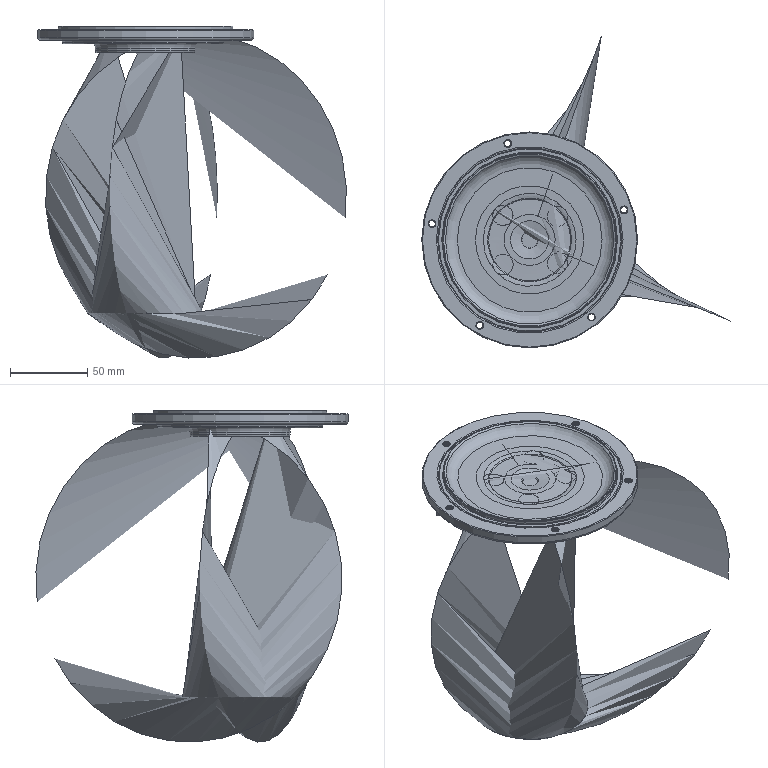NC program | NX | posted with a generic post
Lines 1 to 1953 of 2005, first 1677 of 1941 lines:
N10 G17 G21 G94 G90
(FLOOR_WALL_COPY , TOOL : D63)
N12 T01 M6
N14 G54
N16 G17 G0 G90 X-107.375 Y69.872 S6500 M3
N18 G43 Z30. H1
N20 Z5.
N22 G94 G1 Z2. F1250.
N24 X-101.375
N26 X101.375
N28 Y31.69
N30 X-101.375
N32 Y-6.493
N34 X101.375
N36 Y-44.675
N38 X-101.375
N40 X-107.375
N42 Z5.
N44 G0 Z30.
N46 Y69.872
N48 Z4.
N50 G1 Z1.
N52 X-101.375
N54 X101.375
N56 Y31.69
N58 X-101.375
N60 Y-6.493
N62 X101.375
N64 Y-44.675
N66 X-101.375
N68 X-107.375
N70 Z4.
N72 G0 Z30.
N74 Y69.872
N76 Z3.
N78 G1 Z0.
N80 X-101.375
N82 X101.375
N84 Y31.69
N86 X-101.375
N88 Y-6.493
N90 X101.375
N92 Y-44.675
N94 X-101.375
N96 X-107.375
N98 Z3.
N100 G0 Z30.
N102 M5
(CAVITY_MILL_COPY , TOOL : D10)
N104 T10 M6
N106 G54
N108 G17 G0 G90 X-76.871 Y-18.279 S9500 M3
N110 G43 Z30. H10
N112 Z0.1
N114 G94 G1 Z-0.9 F750.
N116 X-70.871 Y-14.815
N118 G3 X-70.371 Y-13.949 R1.
N120 G1 Y25.577 F3000.
N122 G2 X-25.577 Y70.371 R74.875
N124 G1 X25.577
N126 G2 X70.371 Y25.577 R74.875
N128 G1 Y-25.577
N130 G2 X25.577 Y-70.371 R74.875
N132 G1 X-25.577
N134 G2 X-70.371 Y-25.577 R74.875
N136 G1 Y-13.949
N138 X-63.871
N140 Y24.405
N142 G2 X-24.405 Y63.871 R68.375
N144 G1 X24.405
N146 G2 X63.871 Y24.405 R68.375
N148 G1 Y-24.405
N150 G2 X24.405 Y-63.871 R68.375
N152 G1 X-24.405
N154 G2 X-63.871 Y-24.405 R68.375
N156 G1 Y-13.949
N158 X-57.371
N160 Y23.175
N162 G2 X-23.175 Y57.371 R61.875
N164 G1 X23.175
N166 G2 X57.371 Y23.175 R61.875
N168 G1 Y-23.175
N170 G2 X23.175 Y-57.371 R61.875
N172 G1 X-23.175
N174 G2 X-57.371 Y-23.175 R61.875
N176 G1 Y-13.949
N178 X-50.871
N180 Y21.875
N182 G2 X-21.875 Y50.871 R55.375
N184 G1 X21.875
N186 G2 X50.871 Y21.875 R55.375
N188 G1 Y-21.875
N190 G2 X21.875 Y-50.871 R55.375
N192 G1 X-21.875
N194 G2 X-50.871 Y-21.875 R55.375
N196 G1 Y-13.949
N198 X-44.371
N200 Y20.493
N202 G2 X-20.493 Y44.371 R48.875
N204 G1 X-8.886
N206 Y37.871
N208 G3 X-37.871 Y8.886 R38.9
N210 G1 Y19.011
N212 G2 X-19.011 Y37.871 R42.375
N214 G1 X-8.886
N216 X0. Y39.1
N218 X-8.886 Y37.871
N220 Y44.371
N222 X20.493
N224 G2 X44.371 Y20.493 R48.875
N226 G1 Y8.886
N228 X37.871
N230 G3 X8.886 Y37.871 R38.9
N232 G1 X19.011
N234 G2 X37.871 Y19.011 R42.375
N236 G1 Y8.886
N238 X39.1 Y0.
N240 X37.871 Y8.886
N242 X44.371
N244 Y-20.493
N246 G2 X20.493 Y-44.371 R48.875
N248 G1 X8.886
N250 Y-37.871
N252 G3 X37.871 Y-8.886 R38.9
N254 G1 Y-19.011
N256 G2 X19.011 Y-37.871 R42.375
N258 G1 X8.886
N260 Y-44.371
N262 X-20.493
N264 G2 X-44.371 Y-20.493 R48.875
N266 G1 Y-13.949
N268 X-37.871
N270 Y-8.886
N272 X-39.1 Y0.
N274 X-37.871 Y-8.886
N276 G3 X-8.886 Y-37.871 R38.9
N278 G1 X0. Y-39.1
N280 X-8.886 Y-37.871
N282 X-8.589 Y-36.605
N284 G2 X-36.605 Y8.589 R37.6
N286 X-8.589 Y-36.605 R-37.6
N288 G1 X-8.886 Y-37.871
N290 X-19.011
N292 G2 X-37.871 Y-19.011 R42.375
N294 G1 Y-13.949
N296 G3 X-38.371 Y-13.082 R1.
N298 G1 Z0.1
N300 G0 X-76.871 Y-18.387 Z-0.8
N302 G1 Z-1.8 F750.
N304 X-70.871 Y-14.922
N306 G3 X-70.371 Y-14.056 R1.
N308 G1 Y25.576 F3000.
N310 G2 X-25.576 Y70.371 R74.875
N312 G1 X25.576
N314 G2 X70.371 Y25.576 R74.875
N316 G1 Y-25.576
N318 G2 X25.576 Y-70.371 R74.875
N320 G1 X-25.576
N322 G2 X-70.371 Y-25.576 R74.875
N324 G1 Y-14.056
N326 X-63.871
N328 Y24.405
N330 G2 X-24.405 Y63.871 R68.375
N332 G1 X24.405
N334 G2 X63.871 Y24.405 R68.375
N336 G1 Y-24.405
N338 G2 X24.405 Y-63.871 R68.375
N340 G1 X-24.405
N342 G2 X-63.871 Y-24.405 R68.375
N344 G1 Y-14.056
N346 X-57.371
N348 Y23.174
N350 G2 X-23.174 Y57.371 R61.875
N352 G1 X23.174
N354 G2 X57.371 Y23.174 R61.875
N356 G1 Y-23.174
N358 G2 X23.174 Y-57.371 R61.875
N360 G1 X-23.174
N362 G2 X-57.371 Y-23.174 R61.875
N364 G1 Y-14.056
N366 X-50.871
N368 Y21.875
N370 G2 X-21.875 Y50.871 R55.375
N372 G1 X21.875
N374 G2 X50.871 Y21.875 R55.375
N376 G1 Y-21.875
N378 G2 X21.875 Y-50.871 R55.375
N380 G1 X-21.875
N382 G2 X-50.871 Y-21.875 R55.375
N384 G1 Y-14.056
N386 X-44.371
N388 Y20.493
N390 G2 X-20.493 Y44.371 R48.875
N392 G1 X-9.102
N394 Y37.871
N396 G3 X-37.871 Y9.102 R38.95
N398 G1 Y19.011
N400 G2 X-19.011 Y37.871 R42.375
N402 G1 X-9.102
N404 X0. Y39.12
N406 X-9.102 Y37.871
N408 Y44.371
N410 X20.493
N412 G2 X44.371 Y20.493 R48.875
N414 G1 Y9.102
N416 X37.871
N418 G3 X9.102 Y37.871 R38.95
N420 G1 X19.011
N422 G2 X37.871 Y19.011 R42.375
N424 G1 Y9.102
N426 X39.12 Y0.
N428 X37.871 Y9.102
N430 X44.371
N432 Y-20.493
N434 G2 X20.493 Y-44.371 R48.875
N436 G1 X9.102
N438 Y-37.871
N440 G3 X37.871 Y-9.102 R38.95
N442 G1 Y-19.011
N444 G2 X19.011 Y-37.871 R42.375
N446 G1 X9.102
N448 Y-44.371
N450 X-20.493
N452 G2 X-44.371 Y-20.493 R48.875
N454 G1 Y-14.056
N456 X-37.871
N458 Y-9.102
N460 X-39.12 Y0.
N462 X-37.871 Y-9.102
N464 G3 X-9.102 Y-37.871 R38.95
N466 G1 X0. Y-39.12
N468 X-9.102 Y-37.871
N470 X-8.798 Y-36.607
N472 G2 X-36.607 Y8.798 R37.65
N474 X-8.798 Y-36.607 R-37.65
N476 G1 X-9.102 Y-37.871
N478 X-19.011
N480 G2 X-37.871 Y-19.011 R42.375
N482 G1 Y-14.056
N484 G3 X-38.371 Y-13.19 R1.
N486 G1 Z-0.8
N488 G0 X-76.871 Y-18.388 Z-1.7
N490 G1 Z-2.7 F750.
N492 X-70.871 Y-14.924
N494 G3 X-70.371 Y-14.057 R1.
N496 G1 Y25.576 F3000.
N498 G2 X-25.576 Y70.371 R74.875
N500 G1 X25.576
N502 G2 X70.371 Y25.576 R74.875
N504 G1 Y-25.576
N506 G2 X25.576 Y-70.371 R74.875
N508 G1 X-25.576
N510 G2 X-70.371 Y-25.576 R74.875
N512 G1 Y-14.057
N514 X-63.871
N516 Y24.404
N518 G2 X-24.404 Y63.871 R68.375
N520 G1 X24.404
N522 G2 X63.871 Y24.404 R68.375
N524 G1 Y-24.404
N526 G2 X24.404 Y-63.871 R68.375
N528 G1 X-24.404
N530 G2 X-63.871 Y-24.404 R68.375
N532 G1 Y-14.057
N534 X-57.371
N536 Y23.174
N538 G2 X-23.174 Y57.371 R61.875
N540 G1 X23.174
N542 G2 X57.371 Y23.174 R61.875
N544 G1 Y-23.174
N546 G2 X23.174 Y-57.371 R61.875
N548 G1 X-23.174
N550 G2 X-57.371 Y-23.174 R61.875
N552 G1 Y-14.057
N554 X-50.871
N556 Y21.874
N558 G2 X-21.874 Y50.871 R55.375
N560 G1 X21.874
N562 G2 X50.871 Y21.874 R55.375
N564 G1 Y-21.874
N566 G2 X21.874 Y-50.871 R55.375
N568 G1 X-21.874
N570 G2 X-50.871 Y-21.874 R55.375
N572 G1 Y-14.057
N574 X-44.371
N576 Y20.492
N578 G2 X-20.492 Y44.371 R48.875
N580 G1 X-9.105
N582 Y37.871
N584 G3 X-17.369 Y34.864 R38.951
N586 X-19.724 Y33.588 R38.951
N588 X-21.468 Y32.5 R38.951
N590 X-22.403 Y31.863 R38.951
N592 X-24.645 Y30.163 R38.951
N594 X-30.163 Y24.645 R38.951
N596 X-33.556 Y19.777 R38.951
N598 X-35.962 Y14.962 R38.951
N600 X-36.787 Y12.802 R38.951
N602 X-37.585 Y10.222 R38.951
N604 X-37.871 Y9.105 R38.951
N606 G1 Y19.01
N608 G2 X-19.01 Y37.871 R42.375
N610 G1 X-9.105
N612 X0. Y39.12
N614 X-9.105 Y37.871
N616 Y44.371
N618 X20.492
N620 G2 X44.371 Y20.492 R48.875
N622 G1 Y9.105
N624 X37.871
N626 G3 X13.605 Y36.497 R38.951
N628 X9.105 Y37.871 R38.951
N630 G1 X19.01
N632 G2 X37.871 Y19.01 R42.375
N634 G1 Y9.105
N636 X39.12 Y0.
N638 X37.871 Y9.105
N640 X44.371
N642 Y-20.492
N644 G2 X20.492 Y-44.371 R48.875
N646 G1 X9.105
N648 Y-37.871
N650 G3 X37.871 Y-9.105 R38.951
N652 G1 Y-19.01
N654 G2 X19.01 Y-37.871 R42.375
N656 G1 X9.105
N658 Y-44.371
N660 X-20.492
N662 G2 X-44.371 Y-20.492 R48.875
N664 G1 Y-14.057
N666 X-37.871
N668 Y-9.105
N670 X-39.12 Y0.
N672 X-37.871 Y-9.105
N674 G3 X-9.105 Y-37.871 R38.951
N676 G1 X0. Y-39.12
N678 X-9.105 Y-37.871
N680 X-8.801 Y-36.607
N682 G2 X-29.083 Y-23.911 R37.651
N684 G1 X-29.156 Y-23.822
N686 G2 X-30.8 Y-21.655 R37.651
N688 G1 X-30.9 Y-21.511
N690 G2 X-37.65 Y-0.121 R37.651
N692 X-37.65 Y0.121 R37.651
N694 X16.143 Y34.014 R37.651
N696 G1 X16.243 Y33.967
N698 G2 X-8.801 Y-36.607 R37.651
N700 G1 X-9.105 Y-37.871
N702 X-19.01
N704 G2 X-37.871 Y-19.01 R42.375
N706 G1 Y-14.057
N708 G3 X-38.371 Y-13.191 R1.
N710 G1 Z-1.7
N712 G0 X-76.872 Y-18.597 Z-2.6
N714 G1 Z-3.6 F750.
N716 X-70.872 Y-15.132
N718 G3 X-70.372 Y-14.266 R1.
N720 G1 Y25.575 F3000.
N722 G2 X-25.575 Y70.372 R74.875
N724 G1 X25.575
N726 G2 X70.372 Y25.575 R74.875
N728 G1 Y-25.575
N730 G2 X25.575 Y-70.372 R74.875
N732 G1 X-25.575
N734 G2 X-70.372 Y-25.575 R74.875
N736 G1 Y-14.266
N738 X-63.872
N740 Y24.404
N742 G2 X-24.404 Y63.872 R68.375
N744 G1 X24.404
N746 G2 X63.872 Y24.404 R68.375
N748 G1 Y-24.404
N750 G2 X24.404 Y-63.872 R68.375
N752 G1 X-24.404
N754 G2 X-63.872 Y-24.404 R68.375
N756 G1 Y-14.266
N758 X-57.372
N760 Y23.173
N762 G2 X-23.173 Y57.372 R61.875
N764 G1 X23.173
N766 G2 X57.372 Y23.173 R61.875
N768 G1 Y-23.173
N770 G2 X23.173 Y-57.372 R61.875
N772 G1 X-23.173
N774 G2 X-57.372 Y-23.173 R61.875
N776 G1 Y-14.266
N778 X-50.872
N780 Y21.874
N782 G2 X-21.874 Y50.872 R55.375
N784 G1 X21.874
N786 G2 X50.872 Y21.874 R55.375
N788 G1 Y-21.874
N790 G2 X21.874 Y-50.872 R55.375
N792 G1 X-21.874
N794 G2 X-50.872 Y-21.874 R55.375
N796 G1 Y-14.266
N798 X-44.372
N800 Y20.492
N802 G2 X-20.492 Y44.372 R48.875
N804 G1 X-9.523
N806 Y37.872
N808 G3 X-37.872 Y9.523 R39.051
N810 G1 Y19.01
N812 G2 X-19.01 Y37.872 R42.375
N814 G1 X-9.523
N816 X-4.606 Y38.778
N818 G2 X4.606 Y38.778 R39.051
N820 X4.753 Y39.372 R5.
N822 G1 X-4.753
N824 G2 X-4.606 Y38.778 R5.
N826 G1 X-9.523 Y37.872
N828 Y44.372
N830 X20.492
N832 G2 X44.372 Y20.492 R48.875
N834 G1 Y9.523
N836 X37.872
N838 G3 X9.523 Y37.872 R39.051
N840 G1 X19.01
N842 G2 X37.872 Y19.01 R42.375
N844 G1 Y9.523
N846 X38.778 Y4.606
N848 G2 X38.778 Y-4.606 R39.051
N850 X39.372 Y-4.753 R5.
N852 G1 Y4.753
N854 G2 X38.778 Y4.606 R5.
N856 G1 X37.872 Y9.523
N858 X44.372
N860 Y-20.492
N862 G2 X20.492 Y-44.372 R48.875
N864 G1 X9.523
N866 Y-37.872
N868 G3 X37.872 Y-9.523 R39.051
N870 G1 Y-19.01
N872 G2 X19.01 Y-37.872 R42.375
N874 G1 X9.523
N876 Y-44.372
N878 X-20.492
N880 G2 X-44.372 Y-20.492 R48.875
N882 G1 Y-14.266
N884 X-37.872
N886 Y-9.523
N888 X-38.778 Y-4.606
N890 G2 X-38.778 Y4.606 R39.051
N892 X-39.372 Y4.753 R5.
N894 G1 Y-4.753
N896 G2 X-38.778 Y-4.606 R5.
N898 G1 X-37.872 Y-9.523
N900 G3 X-9.523 Y-37.872 R39.051
N902 G1 X-4.753 Y-39.372
N904 X4.753
N906 G2 X4.606 Y-38.778 R5.
N908 X-4.606 Y-38.778 R39.051
N910 X-4.753 Y-39.372 R5.
N912 G1 X-9.523 Y-37.872
N914 X-9.206 Y-36.611
N916 G2 X-36.611 Y9.206 R37.751
N918 X-9.206 Y-36.611 R-37.751
N920 G1 X-9.523 Y-37.872
N922 X-19.01
N924 G2 X-37.872 Y-19.01 R42.375
N926 G1 Y-14.266
N928 G3 X-38.372 Y-13.4 R1.
N930 G1 Z-2.6
N932 G0 X-76.872 Y-19.041 Z-3.355
N934 G1 Z-4.355 F750.
N936 X-70.872 Y-15.576
N938 G3 X-70.372 Y-14.71 R1.
N940 G1 Y25.575 F3000.
N942 G2 X-25.575 Y70.372 R74.875
N944 G1 X25.575
N946 G2 X70.372 Y25.575 R74.875
N948 G1 Y-25.575
N950 G2 X25.575 Y-70.372 R74.875
N952 G1 X-25.575
N954 G2 X-70.372 Y-25.575 R74.875
N956 G1 Y-14.71
N958 X-63.872
N960 Y24.403
N962 G2 X-24.403 Y63.872 R68.375
N964 G1 X24.403
N966 G2 X63.872 Y24.403 R68.375
N968 G1 Y-24.403
N970 G2 X24.403 Y-63.872 R68.375
N972 G1 X-24.403
N974 G2 X-63.872 Y-24.403 R68.375
N976 G1 Y-14.71
N978 X-57.372
N980 Y23.173
N982 G2 X-23.173 Y57.372 R61.875
N984 G1 X23.173
N986 G2 X57.372 Y23.173 R61.875
N988 G1 Y-23.173
N990 G2 X23.173 Y-57.372 R61.875
N992 G1 X-23.173
N994 G2 X-57.372 Y-23.173 R61.875
N996 G1 Y-14.71
N998 X-50.872
N1000 Y21.873
N1002 G2 X-21.873 Y50.872 R55.375
N1004 G1 X21.873
N1006 G2 X50.872 Y21.873 R55.375
N1008 G1 Y-21.873
N1010 G2 X21.873 Y-50.872 R55.375
N1012 G1 X-21.873
N1014 G2 X-50.872 Y-21.873 R55.375
N1016 G1 Y-14.71
N1018 X-44.372
N1020 Y20.492
N1022 G2 X-20.492 Y44.372 R48.875
N1024 G1 X-10.411
N1026 Y37.872
N1028 G3 X-37.872 Y10.411 R39.277
N1030 G1 Y19.01
N1032 G2 X-19.01 Y37.872 R42.375
N1034 G1 X-10.411
N1036 X-5.516 Y38.888
N1038 G2 X5.516 Y38.888 R39.277
N1040 X5.642 Y39.372 R5.
N1042 G1 X-5.642
N1044 G2 X-5.516 Y38.888 R5.
N1046 G1 X-10.411 Y37.872
N1048 Y44.372
N1050 X20.492
N1052 G2 X44.372 Y20.492 R48.875
N1054 G1 Y10.411
N1056 X37.872
N1058 G3 X10.411 Y37.872 R39.277
N1060 G1 X19.01
N1062 G2 X37.872 Y19.01 R42.375
N1064 G1 Y10.411
N1066 X38.888 Y5.516
N1068 G2 X38.888 Y-5.516 R39.277
N1070 X39.372 Y-5.642 R5.
N1072 G1 Y5.642
N1074 G2 X38.888 Y5.516 R5.
N1076 G1 X37.872 Y10.411
N1078 X44.372
N1080 Y-20.492
N1082 G2 X20.492 Y-44.372 R48.875
N1084 G1 X10.411
N1086 Y-37.872
N1088 G3 X37.872 Y-10.411 R39.277
N1090 G1 Y-19.01
N1092 G2 X19.01 Y-37.872 R42.375
N1094 G1 X10.411
N1096 Y-44.372
N1098 X-20.492
N1100 G2 X-44.372 Y-20.492 R48.875
N1102 G1 Y-14.71
N1104 X-37.872
N1106 Y-10.411
N1108 X-38.888 Y-5.516
N1110 G2 X-38.888 Y5.516 R39.277
N1112 X-39.372 Y5.642 R5.
N1114 G1 Y-5.642
N1116 G2 X-38.888 Y-5.516 R5.
N1118 G1 X-37.872 Y-10.411
N1120 G3 X-10.411 Y-37.872 R39.277
N1122 G1 X-5.642 Y-39.372
N1124 X5.642
N1126 G2 X5.516 Y-38.888 R5.
N1128 X-5.516 Y-38.888 R39.277
N1130 X-5.642 Y-39.372 R5.
N1132 G1 X-10.411 Y-37.872
N1134 X-10.067 Y-36.618
N1136 G2 X-36.618 Y10.067 R37.977
N1138 X-10.067 Y-36.618 R-37.977
N1140 G1 X-10.411 Y-37.872
N1142 X-19.01
N1144 G2 X-37.872 Y-19.01 R42.375
N1146 G1 Y-14.71
N1148 G3 X-38.372 Y-13.844 R1.
N1150 G1 Z-3.355
N1152 G0 X-76.872 Y-19.706 Z-4.111
N1154 G1 Z-5.111 F750.
N1156 X-70.872 Y-16.241
N1158 G3 X-70.372 Y-15.375 R1.
N1160 G1 Y25.574 F3000.
N1162 G2 X-25.574 Y70.372 R74.875
N1164 G1 X25.574
N1166 G2 X70.372 Y25.574 R74.875
N1168 G1 Y-25.574
N1170 G2 X25.574 Y-70.372 R74.875
N1172 G1 X-25.574
N1174 G2 X-70.372 Y-25.574 R74.875
N1176 G1 Y-15.375
N1178 X-63.872
N1180 Y24.403
N1182 G2 X-24.403 Y63.872 R68.375
N1184 G1 X24.403
N1186 G2 X63.872 Y24.403 R68.375
N1188 G1 Y-24.403
N1190 G2 X24.403 Y-63.872 R68.375
N1192 G1 X-24.403
N1194 G2 X-63.872 Y-24.403 R68.375
N1196 G1 Y-15.375
N1198 X-57.372
N1200 Y23.173
N1202 G2 X-23.173 Y57.372 R61.875
N1204 G1 X23.173
N1206 G2 X57.372 Y23.173 R61.875
N1208 G1 Y-23.173
N1210 G2 X23.173 Y-57.372 R61.875
N1212 G1 X-23.173
N1214 G2 X-57.372 Y-23.173 R61.875
N1216 G1 Y-15.375
N1218 X-50.872
N1220 Y21.873
N1222 G2 X-21.873 Y50.872 R55.375
N1224 G1 X21.873
N1226 G2 X50.872 Y21.873 R55.375
N1228 G1 Y-21.873
N1230 G2 X21.873 Y-50.872 R55.375
N1232 G1 X-21.873
N1234 G2 X-50.872 Y-21.873 R55.375
N1236 G1 Y-15.375
N1238 X-44.372
N1240 Y20.491
N1242 G2 X-20.491 Y44.372 R48.875
N1244 G1 X-11.742
N1246 Y37.872
N1248 G3 X-37.872 Y11.742 R39.65
N1250 G1 X-39.267 Y6.206
N1252 X-37.872 Y11.742
N1254 Y19.009
N1256 G2 X-19.009 Y37.872 R42.375
N1258 G1 X-11.742
N1260 X-6.206 Y39.267
N1262 X-11.742 Y37.872
N1264 Y44.372
N1266 X20.491
N1268 G2 X44.372 Y20.491 R48.875
N1270 G1 Y11.742
N1272 X37.872
N1274 G3 X11.742 Y37.872 R39.65
N1276 G1 X6.206 Y39.267
N1278 X11.742 Y37.872
N1280 X19.009
N1282 G2 X37.872 Y19.009 R42.375
N1284 G1 Y11.742
N1286 X39.267 Y6.206
N1288 X37.872 Y11.742
N1290 X44.372
N1292 Y-20.491
N1294 G2 X20.491 Y-44.372 R48.875
N1296 G1 X11.742
N1298 Y-37.872
N1300 G3 X37.872 Y-11.742 R39.65
N1302 G1 X39.267 Y-6.206
N1304 X37.872 Y-11.742
N1306 Y-19.009
N1308 G2 X19.009 Y-37.872 R42.375
N1310 G1 X11.742
N1312 X6.206 Y-39.267
N1314 X11.742 Y-37.872
N1316 Y-44.372
N1318 X-20.491
N1320 G2 X-44.372 Y-20.491 R48.875
N1322 G1 Y-15.375
N1324 X-37.872
N1326 Y-11.742
N1328 X-39.267 Y-6.206
N1330 X-37.872 Y-11.742
N1332 G3 X-11.742 Y-37.872 R39.65
N1334 G1 X-6.206 Y-39.267
N1336 X-11.742 Y-37.872
N1338 X-11.357 Y-36.63
N1340 G2 X-36.63 Y11.357 R38.35
N1342 X-11.357 Y-36.63 R-38.35
N1344 G1 X-11.742 Y-37.872
N1346 X-19.009
N1348 G2 X-37.872 Y-19.009 R42.375
N1350 G1 Y-15.375
N1352 G3 X-38.372 Y-14.509 R1.
N1354 G1 Z-4.111
N1356 G0 X-76.198 Y-23.956 Z-4.866
N1358 G1 Z-5.866 F750.
N1360 X-70.872 Y-20.882
N1362 G3 X-70.372 Y-20.016 R1.
N1364 G1 Y25.574 F3000.
N1366 G2 X-25.574 Y70.372 R74.875
N1368 G1 X25.574
N1370 G2 X70.372 Y25.574 R74.875
N1372 G1 Y-25.574
N1374 G2 X25.574 Y-70.372 R74.875
N1376 G1 X-25.574
N1378 G2 X-70.372 Y-25.574 R74.875
N1380 G1 Y-20.016
N1382 X-63.872
N1384 Y24.403
N1386 G2 X-24.403 Y63.872 R68.375
N1388 G1 X-16.859
N1390 Y57.372
N1392 G3 X-57.372 Y16.859 R59.798
N1394 G1 X-58.776 Y11.531
N1396 X-57.372 Y16.859
N1398 Y23.172
N1400 G2 X-23.172 Y57.372 R61.875
N1402 G1 X-16.859
N1404 X-11.531 Y58.776
N1406 X-16.859 Y57.372
N1408 Y63.872
N1410 X24.403
N1412 G2 X63.872 Y24.403 R68.375
N1414 G1 Y16.859
N1416 X57.372
N1418 G3 X16.859 Y57.372 R59.798
N1420 G1 X11.531 Y58.776
N1422 X16.859 Y57.372
N1424 X23.172
N1426 G2 X57.372 Y23.172 R61.875
N1428 G1 Y16.859
N1430 X58.776 Y11.531
N1432 X57.372 Y16.859
N1434 X63.872
N1436 Y-24.403
N1438 G2 X24.403 Y-63.872 R68.375
N1440 G1 X16.859
N1442 Y-57.372
N1444 G3 X57.372 Y-16.859 R59.798
N1446 G1 X58.776 Y-11.531
N1448 X57.372 Y-16.859
N1450 Y-23.172
N1452 G2 X23.172 Y-57.372 R61.875
N1454 G1 X16.859
N1456 X11.531 Y-58.776
N1458 X16.859 Y-57.372
N1460 Y-63.872
N1462 X-24.403
N1464 G2 X-63.872 Y-24.403 R68.375
N1466 G1 Y-20.016
N1468 X-57.372
N1470 Y-16.859
N1472 X-58.776 Y-11.531
N1474 X-57.372 Y-16.859
N1476 G3 X-16.859 Y-57.372 R59.798
N1478 G1 X-11.531 Y-58.776
N1480 X-16.859 Y-57.372
N1482 X-16.492 Y-56.125
N1484 G2 X-56.125 Y16.492 R58.498
N1486 X-16.492 Y-56.125 R-58.498
N1488 G1 X-16.859 Y-57.372
N1490 X-23.172
N1492 G2 X-57.372 Y-23.172 R61.875
N1494 G1 Y-20.016
N1496 G3 X-57.872 Y-19.15 R1.
N1498 G1 Z-4.866
N1500 G0 X-75.981 Y-24.636 Z-5.622
N1502 G1 Z-6.622 F750.
N1504 X-70.872 Y-21.687
N1506 G3 X-70.372 Y-20.821 R1.
N1508 G1 Y25.573 F3000.
N1510 G2 X-25.573 Y70.372 R74.875
N1512 G1 X25.573
N1514 G2 X70.372 Y25.573 R74.875
N1516 G1 Y-25.573
N1518 G2 X25.573 Y-70.372 R74.875
N1520 G1 X-25.573
N1522 G2 X-70.372 Y-25.573 R74.875
N1524 G1 Y-20.821
N1526 X-63.872
N1528 Y24.402
N1530 G2 X-24.402 Y63.872 R68.375
N1532 G1 X-18.47
N1534 Y57.372
N1536 G3 X-57.372 Y18.47 R60.272
N1538 G1 X-58.817 Y13.423
N1540 X-57.372 Y18.47
N1542 Y23.172
N1544 G2 X-23.172 Y57.372 R61.875
N1546 G1 X-18.47
N1548 X-13.423 Y58.817
N1550 X-18.47 Y57.372
N1552 Y63.872
N1554 X24.402
N1556 G2 X63.872 Y24.402 R68.375
N1558 G1 Y18.47
N1560 X57.372
N1562 G3 X18.47 Y57.372 R60.272
N1564 G1 X13.423 Y58.817
N1566 X18.47 Y57.372
N1568 X23.172
N1570 G2 X57.372 Y23.172 R61.875
N1572 G1 Y18.47
N1574 X58.817 Y13.423
N1576 X57.372 Y18.47
N1578 X63.872
N1580 Y-24.402
N1582 G2 X24.402 Y-63.872 R68.375
N1584 G1 X18.47
N1586 Y-57.372
N1588 G3 X57.372 Y-18.47 R60.272
N1590 G1 X58.817 Y-13.423
N1592 X57.372 Y-18.47
N1594 Y-23.172
N1596 G2 X23.172 Y-57.372 R61.875
N1598 G1 X18.47
N1600 X13.423 Y-58.817
N1602 X18.47 Y-57.372
N1604 Y-63.872
N1606 X-24.402
N1608 G2 X-63.872 Y-24.402 R68.375
N1610 G1 Y-20.821
N1612 X-57.372
N1614 Y-18.47
N1616 X-58.817 Y-13.423
N1618 X-57.372 Y-18.47
N1620 G3 X-18.47 Y-57.372 R60.272
N1622 G1 X-13.423 Y-58.817
N1624 X-18.47 Y-57.372
N1626 X-18.071 Y-56.135
N1628 G2 X-56.135 Y18.071 R58.972
N1630 X-18.071 Y-56.135 R-58.972
N1632 G1 X-18.47 Y-57.372
N1634 X-23.172
N1636 G2 X-57.372 Y-23.172 R61.875
N1638 G1 Y-20.821
N1640 G3 X-57.872 Y-19.955 R1.
N1642 G1 Z-5.622
N1644 G0 X-75.943 Y-24.754 Z-6.414
N1646 G1 Z-7.414 F750.
N1648 X-70.872 Y-21.827
N1650 G3 X-70.372 Y-20.96 R1.
N1652 G1 Y25.573 F3000.
N1654 G2 X-25.573 Y70.372 R74.875
N1656 G1 X25.573
N1658 G2 X70.372 Y25.573 R74.875
N1660 G1 Y-25.573
N1662 G2 X25.573 Y-70.372 R74.875
N1664 G1 X-25.573
N1666 G2 X-70.372 Y-25.573 R74.875
N1668 G1 Y-20.96
N1670 X-63.872
N1672 Y24.402
N1674 G2 X-24.402 Y63.872 R68.375
N1676 G1 X-18.75
N1678 Y57.372
N1680 G3 X-57.372 Y18.75 R60.359
N1682 G1 X-58.824 Y13.743
N1684 X-57.372 Y18.75
N1686 Y23.171
N1688 G2 X-23.171 Y57.372 R61.875
N1690 G1 X-18.75
N1692 X-13.743 Y58.824
N1694 X-18.75 Y57.372
N1696 Y63.872
N1698 X24.402
N1700 G2 X63.872 Y24.402 R68.375
N1702 G1 Y18.75
N1704 X57.372
N1706 G3 X18.75 Y57.372 R60.359
N1708 G1 X13.743 Y58.824
N1710 X18.75 Y57.372
N1712 X23.171
N1714 G2 X57.372 Y23.171 R61.875
N1716 G1 Y18.75
N1718 X58.824 Y13.743
N1720 X57.372 Y18.75
N1722 X63.872
N1724 Y-24.402
N1726 G2 X24.402 Y-63.872 R68.375
N1728 G1 X18.75
N1730 Y-57.372
N1732 G3 X57.372 Y-18.75 R60.359
N1734 G1 X58.824 Y-13.743
N1736 X57.372 Y-18.75
N1738 Y-23.171
N1740 G2 X23.171 Y-57.372 R61.875
N1742 G1 X18.75
N1744 X13.743 Y-58.824
N1746 X18.75 Y-57.372
N1748 Y-63.872
N1750 X-24.402
N1752 G2 X-63.872 Y-24.402 R68.375
N1754 G1 Y-20.96
N1756 X-57.372
N1758 Y-18.75
N1760 X-58.824 Y-13.743
N1762 X-57.372 Y-18.75
N1764 G3 X-18.75 Y-57.372 R60.359
N1766 G1 X-13.743 Y-58.824
N1768 X-18.75 Y-57.372
N1770 X-18.346 Y-56.137
N1772 G2 X-56.137 Y18.346 R59.059
N1774 X-18.346 Y-56.137 R-59.059
N1776 G1 X-18.75 Y-57.372
N1778 X-23.171
N1780 G2 X-57.372 Y-23.171 R61.875
N1782 G1 Y-20.96
N1784 G3 X-57.872 Y-20.094 R1.
N1786 G1 Z-6.414
N1788 G0 X-75.626 Y-25.705 Z-6.957
N1790 G1 Z-7.957 F750.
N1792 X-70.873 Y-22.961
N1794 G3 X-70.373 Y-22.095 R1.
N1796 G1 Y25.573 F3000.
N1798 G2 X-25.573 Y70.373 R74.875
N1800 G1 X25.573
N1802 G2 X70.373 Y25.573 R74.875
N1804 G1 Y-25.573
N1806 G2 X25.573 Y-70.373 R74.875
N1808 G1 X-25.573
N1810 G2 X-70.373 Y-25.573 R74.875
N1812 G1 Y-22.095
N1814 X-63.873
N1816 Y24.401
N1818 G2 X-24.401 Y63.873 R68.375
N1820 G1 X-21.018
N1822 Y57.373
N1824 G3 X-57.373 Y21.018 R61.101
N1826 G1 Y23.171
N1828 G2 X-23.171 Y57.373 R61.875
N1830 G1 X-21.018
N1832 Y63.873
N1834 X24.401
N1836 G2 X63.873 Y24.401 R68.375
N1838 G1 Y21.018
N1840 X57.373
N1842 G3 X21.018 Y57.373 R61.101
N1844 G1 X23.171
N1846 G2 X57.373 Y23.171 R61.875
N1848 G1 Y21.018
N1850 X63.873
N1852 Y-24.401
N1854 G2 X24.401 Y-63.873 R68.375
N1856 G1 X21.018
N1858 Y-57.373
N1860 G3 X57.373 Y-21.018 R61.101
N1862 G1 Y-23.171
N1864 G2 X23.171 Y-57.373 R61.875
N1866 G1 X21.018
N1868 Y-63.873
N1870 X-24.401
N1872 G2 X-63.873 Y-24.401 R68.375
N1874 G1 Y-22.095
N1876 X-57.373
N1878 Y-21.018
N1880 G3 X-21.018 Y-57.373 R61.101
N1882 G1 X-20.571 Y-56.152
N1884 G2 X-56.152 Y20.571 R59.801
N1886 X-20.571 Y-56.152 R-59.801
N1888 G1 X-21.018 Y-57.373
N1890 X-23.171
N1892 G2 X-57.373 Y-23.171 R61.875
N1894 G1 Y-22.095
N1896 G3 X-57.873 Y-21.229 R1.
N1898 G1 Z-6.957
N1900 G0 X-75.923 Y-24.812 Z-7.17
N1902 G1 Z-8.17 F750.
N1904 X-70.684 Y-23.1
N1906 G3 X-70.467 Y-22.124 R1.
N1908 G2 X-22.124 Y70.467 R73.858 F3000.
N1910 X-70.467 Y-22.124 R-73.858
N1912 G3 X-71.203 Y-21.448 R1.
N1914 G1 X-76.873 Y-20.183
N1916 Z-7.17
N1918 G0 Y-29.25 Z-7.875
N1920 G1 Z-8.875 F750.
N1922 X-71.442 Y-23.338
N1924 G3 X-71.224 Y-22.362 R1.
N1926 G2 X-22.362 Y71.224 R74.652 F3000.
N1928 X-71.224 Y-22.362 R-74.652
N1930 G3 X-71.961 Y-21.686 R1.
N1932 G1 X-76.873 Y-20.59
N1934 Z-7.875
N1936 G0 Z30.
N1938 X29.473 Y-30.052
N1940 Z-4.111
N1942 G1 X31.613 Y-27.871 Z-4.271 F750.
N1944 X34.39 Y-24.361 Z-4.506
N1946 X36.78 Y-20.576 Z-4.74
N1948 X38.755 Y-16.559 Z-4.975
N1950 X40.293 Y-12.356 Z-5.209
N1952 X41.376 Y-8.013 Z-5.444
N1954 X41.862 Y-4.87 Z-5.61
N1956 X42.114 Y-1.59 Z-5.783
N1958 Y0. Z-5.866
N1960 G3 X0. Y42.114 R42.114 F3000.
N1962 X42.114 Y0. R-42.114
N1964 G1 X46.614
N1966 G3 X-29.207 Y-36.33 R-46.614
N1968 G1 X-24.386 Y-30.333
N1970 G2 X-30.333 Y24.386 R38.92
N1972 X-24.386 Y-30.333 R-38.92
N1974 G1 X-29.207 Y-36.33
N1976 G3 X46.614 Y0. R46.614
N1978 X46.114 Y0.866 R1.
N1980 G1 Z-4.866
N1982 G0 Z30.
N1984 X-29.656 Y26.524
N1986 Z-4.866
N1988 G1 X-28.742 Y27.586 Z-4.94 F750.
N1990 X-25.612 Y30.514 Z-5.164
N1992 X-22.186 Y33.088 Z-5.389
N1994 X-19.554 Y34.709 Z-5.551
N1996 X-16.179 Y36.405 Z-5.749
N1998 X-12.658 Y37.774 Z-5.947
N2000 X-9.024 Y38.803 Z-6.145
N2002 X-5.309 Y39.483 Z-6.343
N2004 X-1.546 Y39.808 Z-6.541
N2006 X0. Z-6.622
N2008 G2 X39.808 Y0. R39.808 F3000.
N2010 X0. Y39.808 R-39.808
N2012 G1 Y43.854
N2014 G3 X-43.854 Y0. R43.854
N2016 X0. Y43.854 R-43.854
N2018 X-0.866 Y43.354 R1.
N2020 G1 Z-5.622
N2022 G0 Z30.
N2024 X4.327 Y2.316
N2026 Z1.
N2028 G1 X4.229 Y2.553 Z0.987 F750.
N2030 X3.264 Y3.708 Z0.908
N2032 X1.997 Y4.519 Z0.829
N2034 X0.544 Y4.91 Z0.75
N2036 X-0.544 Z0.693
N2038 X-1.385 Y4.742 Z0.648
N2040 X-2.185 Y4.43 Z0.603
N2042 X-3.101 Y3.845 Z0.546
N2044 X-4.102 Y2.752 Z0.468
N2046 X-4.734 Y1.411 Z0.391
N2048 X-4.94 Y-0.057 Z0.313
N2050 X-4.7 Y-1.52 Z0.235
N2052 X-4.038 Y-2.846 Z0.158
N2054 X-3.011 Y-3.916 Z0.08
N2056 X-2.082 Y-4.48 Z0.023
N2058 X-0.743 Y-4.884 Z-0.05
N2060 X0.654 Y-4.896 Z-0.124
N2062 X2. Y-4.517 Z-0.197
N2064 X3.185 Y-3.776 Z-0.27
N2066 X4.116 Y-2.732 Z-0.343
N2068 X4.716 Y-1.47 Z-0.417
N2070 X4.924 Y-0.403 Z-0.474
N2072 X4.939 Y0.083 Z-0.499
N2074 X4.802 Y1.161 Z-0.556
N2076 X4.229 Y2.553 Z-0.635
N2078 X3.264 Y3.708 Z-0.714
N2080 X1.997 Y4.519 Z-0.793
N2082 X0.544 Y4.91 Z-0.872
N2084 X0. Z-0.9
N2086 Y0.41
N2088 G3 X-0.41 Y0. R0.41 F3000.
N2090 X0. Y0.41 R-0.41
N2092 G1 Y4.91
N2094 G3 X-4.91 Y0. R4.91
N2096 X0. Y4.91 R-4.91
N2098 G1 Y11.41
N2100 G3 X-11.41 Y0. R11.41
N2102 X0. Y11.41 R-11.41
N2104 G1 Y17.91
N2106 G3 X-17.91 Y0. R17.91
N2108 X0. Y17.91 R-17.91
N2110 G1 Y24.41
N2112 G3 X-24.41 Y0. R24.41
N2114 X0. Y24.41 R-24.41
N2116 X-0.866 Y23.91 R1.
N2118 G1 Z0.1
N2120 G0 Z30.
N2122 X4.327 Y2.316
N2124 Z0.1
N2126 G1 X4.229 Y2.553 Z0.087 F750.
N2128 X3.264 Y3.708 Z0.008
N2130 X1.997 Y4.519 Z-0.071
N2132 X0.544 Y4.91 Z-0.15
N2134 X-0.544 Z-0.207
N2136 X-1.385 Y4.742 Z-0.252
N2138 X-2.185 Y4.43 Z-0.297
N2140 X-3.101 Y3.845 Z-0.354
N2142 X-4.102 Y2.752 Z-0.432
N2144 X-4.734 Y1.411 Z-0.509
N2146 X-4.94 Y-0.057 Z-0.587
N2148 X-4.7 Y-1.52 Z-0.665
N2150 X-4.038 Y-2.846 Z-0.742
N2152 X-3.011 Y-3.916 Z-0.82
N2154 X-2.082 Y-4.48 Z-0.877
N2156 X-0.743 Y-4.884 Z-0.95
N2158 X0.654 Y-4.896 Z-1.024
N2160 X2. Y-4.517 Z-1.097
N2162 X3.185 Y-3.776 Z-1.17
N2164 X4.116 Y-2.732 Z-1.243
N2166 X4.716 Y-1.47 Z-1.317
N2168 X4.924 Y-0.403 Z-1.374
N2170 X4.939 Y0.083 Z-1.399
N2172 X4.802 Y1.161 Z-1.456
N2174 X4.229 Y2.553 Z-1.535
N2176 X3.264 Y3.708 Z-1.614
N2178 X1.997 Y4.519 Z-1.693
N2180 X0.544 Y4.91 Z-1.772
N2182 X0. Z-1.8
N2184 Y0.41
N2186 G3 X-0.41 Y0. R0.41 F3000.
N2188 X0. Y0.41 R-0.41
N2190 G1 Y4.91
N2192 G3 X-4.91 Y0. R4.91
N2194 X0. Y4.91 R-4.91
N2196 G1 Y11.41
N2198 G3 X-11.41 Y0. R11.41
N2200 X0. Y11.41 R-11.41
N2202 G1 Y17.91
N2204 G3 X-17.91 Y0. R17.91
N2206 X0. Y17.91 R-17.91
N2208 G1 Y24.41
N2210 G3 X-24.41 Y0. R24.41
N2212 X0. Y24.41 R-24.41
N2214 X-0.866 Y23.91 R1.
N2216 G1 Z-0.8
N2218 G0 X4.327 Y2.316
N2220 G1 X4.229 Y2.553 Z-0.813 F750.
N2222 X3.264 Y3.708 Z-0.892
N2224 X1.997 Y4.519 Z-0.971
N2226 X0.544 Y4.91 Z-1.05
N2228 X-0.544 Z-1.107
N2230 X-1.385 Y4.742 Z-1.152
N2232 X-2.185 Y4.43 Z-1.197
N2234 X-3.101 Y3.845 Z-1.254
N2236 X-4.102 Y2.752 Z-1.332
N2238 X-4.734 Y1.411 Z-1.409
N2240 X-4.94 Y-0.057 Z-1.487
N2242 X-4.7 Y-1.52 Z-1.565
N2244 X-4.038 Y-2.846 Z-1.642
N2246 X-3.011 Y-3.916 Z-1.72
N2248 X-2.082 Y-4.48 Z-1.777
N2250 X-0.743 Y-4.884 Z-1.85
N2252 X0.654 Y-4.896 Z-1.924
N2254 X2. Y-4.517 Z-1.997
N2256 X3.185 Y-3.776 Z-2.07
N2258 X4.116 Y-2.732 Z-2.143
N2260 X4.716 Y-1.47 Z-2.217
N2262 X4.924 Y-0.403 Z-2.274
N2264 X4.939 Y0.083 Z-2.299
N2266 X4.802 Y1.161 Z-2.356
N2268 X4.229 Y2.553 Z-2.435
N2270 X3.264 Y3.708 Z-2.514
N2272 X1.997 Y4.519 Z-2.593
N2274 X0.544 Y4.91 Z-2.672
N2276 X0. Z-2.7
N2278 Y0.41
N2280 G3 X-0.41 Y0. R0.41 F3000.
N2282 X0. Y0.41 R-0.41
N2284 G1 Y4.91
N2286 G3 X-4.91 Y0. R4.91
N2288 X0. Y4.91 R-4.91
N2290 G1 Y11.41
N2292 G3 X-11.41 Y0. R11.41
N2294 X0. Y11.41 R-11.41
N2296 G1 Y17.91
N2298 G3 X-17.91 Y0. R17.91
N2300 X0. Y17.91 R-17.91
N2302 G1 Y24.41
N2304 G3 X-24.41 Y0. R24.41
N2306 X0. Y24.41 R-24.41
N2308 X-0.866 Y23.91 R1.
N2310 G1 Z-1.7
N2312 G0 X0.808 Y4.446
N2314 G1 X0.76 Y4.462 Z-1.703 F750.
N2316 X-0.581 Y4.489 Z-1.773
N2318 X-1.872 Y4.121 Z-1.843
N2320 X-2.763 Y3.585 Z-1.898
N2322 X-3.609 Y2.731 Z-1.961
N2324 X-4.201 Y1.685 Z-2.024
N2326 X-4.496 Y0.52 Z-2.087
N2328 Y-0.52 Z-2.141
N2330 X-4.221 Y-1.634 Z-2.201
N2332 X-3.675 Y-2.642 Z-2.262
N2334 X-2.893 Y-3.481 Z-2.322
N2336 X-2.021 Y-4.05 Z-2.376
N2338 X-0.839 Y-4.448 Z-2.442
N2340 X0.406 Y-4.508 Z-2.507
N2342 X1.621 Y-4.226 Z-2.572
N2344 X2.713 Y-3.623 Z-2.638
N2346 X3.599 Y-2.745 Z-2.703
N2348 X4.211 Y-1.659 Z-2.768
N2350 X4.479 Y-0.654 Z-2.823
N2352 X4.526 Y-0.083 Z-2.853
N2354 X4.425 Y0.952 Z-2.907
N2356 X3.951 Y2.208 Z-2.978
N2358 X3.131 Y3.269 Z-3.048
N2360 X2.035 Y4.043 Z-3.118
N2362 X0.76 Y4.462 Z-3.189
N2364 X-0.581 Y4.489 Z-3.259
N2366 X-1.872 Y4.121 Z-3.329
N2368 X-2.763 Y3.585 Z-3.384
N2370 X-3.609 Y2.731 Z-3.447
N2372 X-4.201 Y1.685 Z-3.51
N2374 X-4.496 Y0.52 Z-3.573
N2376 Y0. Z-3.6
N2378 G3 X0. Y-4.496 R4.496 F3000.
N2380 X-4.496 Y0. R-4.496
N2382 G1 X-10.996
N2384 G3 X0. Y-10.996 R10.996
N2386 X-10.996 Y0. R-10.996
N2388 G1 X-17.496
N2390 G3 X0. Y-17.496 R17.496
N2392 X-17.496 Y0. R-17.496
N2394 G1 X-23.996
N2396 G3 X0. Y-23.996 R23.996
N2398 X-23.996 Y0. R-23.996
N2400 X-23.496 Y-0.866 R1.
N2402 G1 Z-2.6
N2404 G0 X-0.75 Y-5.464
N2406 G1 X-0.579 Y-5.647 Z-2.613 F750.
N2408 X0. Y-6.449 Z-2.665
N2410 X0.191 Y-6.187 Z-2.682
N2412 X0.845 Y-5.367 Z-2.737
N2414 X1.34 Y-4.839 Z-2.775
N2416 X2.068 Y-4.066 Z-2.831
N2418 X3.257 Y-3.065 Z-2.912
N2420 X4.055 Y-1.886 Z-2.987
N2422 X4.442 Y-0.517 Z-3.061
N2424 Y0.517 Z-3.115
N2426 X4.098 Y1.791 Z-3.185
N2428 X3.397 Y2.909 Z-3.254
N2430 X2.4 Y3.774 Z-3.323
N2432 X1.195 Y4.31 Z-3.392
N2434 X-0.115 Y4.471 Z-3.461
N2436 X-1.414 Y4.243 Z-3.53
N2438 X-2.351 Y3.804 Z-3.584
N2440 X-3.361 Y2.95 Z-3.654
N2442 X-4.077 Y1.838 Z-3.723
N2444 X-4.436 Y0.565 Z-3.792
N2446 X-4.408 Y-0.757 Z-3.862
N2448 X-3.994 Y-2.013 Z-3.931
N2450 X-3.23 Y-3.093 Z-4.
N2452 X-2.069 Y-4.053 Z-4.079
N2454 X-0.579 Y-5.647 Z-4.194
N2456 X0. Y-6.449 Z-4.245
N2458 X0.191 Y-6.187 Z-4.262
N2460 X0.845 Y-5.367 Z-4.317
N2462 X1.34 Y-4.839 Z-4.355
N2464 G2 X2.861 Y-3.398 R17.906 F3000.
N2466 G3 X-2.832 Y-3.423 R-4.442
N2468 G2 X0. Y-6.449 R16.295
N2470 X0.393 Y-5.934 R15.538
N2472 X1.34 Y-4.839 R17.906
N2474 G1 X6.08 Y-9.288
N2476 G2 X7.048 Y-8.37 R11.406
N2478 G3 X-6.975 Y-8.431 R-10.942
N2480 G2 X-4.062 Y-12.501 R9.795
N2482 X-3.506 Y-15.527 R8.53
N2484 G1 Y-19.95
N2486 G3 X3.506 Y-19.95 R20.256
N2488 G1 Y-15.52
N2490 G2 X5.476 Y-9.985 R9.038
N2492 X6.08 Y-9.288 R11.406
N2494 G3 X6.202 Y-9.06 R0.5
N2496 G1 Z-3.355
N2498 G0 X3.531 Y2.625
N2500 G1 X3.504 Y2.671 Z-3.358 F750.
N2502 X2.674 Y3.502 Z-3.42
N2504 X1.654 Y4.084 Z-3.481
N2506 X0.517 Y4.376 Z-3.543
N2508 X-0.51 Y4.377 Z-3.597
N2510 X-1.402 Y4.177 Z-3.645
N2512 X-2.33 Y3.739 Z-3.698
N2514 X-3.331 Y2.884 Z-3.767
N2516 X-4.035 Y1.77 Z-3.836
N2518 X-4.378 Y0.499 Z-3.905
N2520 X-4.33 Y-0.817 Z-3.974
N2522 X-3.895 Y-2.061 Z-4.043
N2524 X-3.112 Y-3.12 Z-4.112
N2526 X-2.709 Y-3.437 Z-4.139
N2528 X-1.916 Y-4.066 Z-4.192
N2530 X-0.634 Y-5.342 Z-4.287
N2532 X-0.002 Y-6.131 Z-4.34
N2534 X0.627 Y-5.346 Z-4.393
N2536 X1.914 Y-4.065 Z-4.488
N2538 X2.703 Y-3.442 Z-4.541
N2540 X3.107 Y-3.125 Z-4.568
N2542 X3.723 Y-2.357 Z-4.619
N2544 X4.153 Y-1.472 Z-4.671
N2546 X4.376 Y-0.513 Z-4.722
N2548 Y0. Z-4.749
N2550 Y0.513 Z-4.776
N2552 X4.085 Y1.651 Z-4.838
N2554 X3.504 Y2.671 Z-4.899
N2556 X2.674 Y3.502 Z-4.961
N2558 X1.654 Y4.084 Z-5.022
N2560 X0.517 Y4.376 Z-5.084
N2562 X0.004 Z-5.111
N2564 G3 X-2.709 Y-3.437 R4.376 F3000.
N2566 G2 X-0.002 Y-6.131 R17.035
N2568 X2.703 Y-3.442 R16.842
N2570 G3 X0.004 Y4.376 R4.376
N2572 G1 X0.009 Y10.876
N2574 G3 X-6.732 Y-8.543 R10.876
N2576 G2 X-4.127 Y-11.595 R10.535
N2578 X-3.07 Y-15.682 R8.675
N2580 G1 Y-19.581
N2582 G3 X3.07 Y-19.581 R19.82
N2584 G1 Y-15.675
N2586 G2 X4.638 Y-10.778 R8.641
N2588 X6.732 Y-8.543 R10.342
N2590 G3 X0.009 Y10.876 R10.876
N2592 X-0.858 Y10.377 R1.
N2594 G1 Z-4.111
N2596 G0 X-2.444 Y-3.542
N2598 G1 X-1.805 Y-3.997 Z-4.152 F750.
N2600 X-0.654 Y-5.024 Z-4.233
N2602 X-0.007 Y-5.746 Z-4.284
N2604 X0.552 Y-5.125 Z-4.327
N2606 X1.178 Y-4.568 Z-4.371
N2608 X1.375 Y-4.393 Z-4.385
N2610 X1.578 Y-4.225 Z-4.399
N2612 X2.48 Y-3.52 Z-4.459
N2614 X2.896 Y-3.227 Z-4.486
N2616 X3.639 Y-2.358 Z-4.545
N2618 X4.128 Y-1.325 Z-4.605
N2620 X4.331 Y-0.2 Z-4.665
N2622 X4.294 Y0.308 Z-4.692
N2624 X4.258 Y0.816 Z-4.719
N2626 X3.83 Y2.03 Z-4.786
N2628 X3.065 Y3.065 Z-4.854
N2630 X2.03 Y3.83 Z-4.921
N2632 X0.816 Y4.258 Z-4.988
N2634 X-0.47 Y4.31 Z-5.056
N2636 X-1.715 Y3.981 Z-5.123
N2638 X-2.597 Y3.472 Z-5.177
N2640 X-3.479 Y2.587 Z-5.242
N2642 X-4.072 Y1.488 Z-5.308
N2644 X-4.327 Y0.265 Z-5.373
N2646 X-4.223 Y-0.98 Z-5.439
N2648 X-3.768 Y-2.144 Z-5.504
N2650 X-3.001 Y-3.129 Z-5.57
N2652 X-2.594 Y-3.436 Z-5.596
N2654 X-1.805 Y-3.997 Z-5.647
N2656 X-0.654 Y-5.024 Z-5.728
N2658 X-0.007 Y-5.746 Z-5.779
N2660 X0.552 Y-5.125 Z-5.822
N2662 X1.176 Y-4.57 Z-5.866
N2664 X1.178 Y-4.568 F3000.
N2666 G2 X1.578 Y-4.225 R15.021
N2668 G1 X2.48 Y-3.52
N2670 G3 X4.294 Y0.308 R4.305
N2672 X-2.594 Y-3.436 R-4.305
N2674 G2 X-0.007 Y-5.746 R15.619
N2676 X1.176 Y-4.57 R15.021
N2678 G1 X5.495 Y-9.428
N2680 G2 X5.671 Y-9.276 R8.521
N2682 G1 X6.408 Y-8.7
N2684 G3 X-6.409 Y-8.7 R-10.805
N2686 G2 X-3.351 Y-12.368 R9.119
N2688 X-2.634 Y-15.704 R8.067
N2690 G1 Y-19.204
N2692 G3 X2.634 Y-19.204 R19.384
N2694 G1 Y-15.7
N2696 G2 X5.495 Y-9.428 R8.521
N2698 G3 X5.637 Y-9.211 R0.5
N2700 G1 Z-4.866
N2702 G0 X-2.198 Y-17.058
N2704 G1 Y-18.82 Z-4.959 F750.
N2706 X-1.138 Y-18.944 Z-5.014
N2708 X1.138 Z-5.134
N2710 X2.198 Y-18.82 Z-5.19
N2712 Y-15.586 Z-5.359
N2714 X2.202 Y-14.877 Z-5.396
N2716 X2.435 Y-13.536 Z-5.468
N2718 X2.882 Y-12.249 Z-5.539
N2720 X3.222 Y-11.627 Z-5.576
N2722 X2.402 Y-11.855 Z-5.621
N2724 X0.803 Y-12.069 Z-5.705
N2726 X-0.81 Y-12.068 Z-5.79
N2728 X-2.409 Y-11.853 Z-5.874
N2730 X-3.229 Y-11.626 Z-5.919
N2732 X-2.888 Y-12.239 Z-5.956
N2734 X-2.433 Y-13.533 Z-6.028
N2736 X-2.199 Y-14.885 Z-6.1
N2738 X-2.198 Y-15.587 Z-6.136
N2740 Y-18.82 Z-6.306
N2742 X-1.138 Y-18.944 Z-6.362
N2744 X1.138 Z-6.481
N2746 X2.198 Y-18.82 Z-6.537
N2748 Y-17.203 Z-6.622
N2750 Y-15.586 F3000.
N2752 G2 X3.222 Y-11.627 R8.362
N2754 X-3.229 Y-11.626 R12.066
N2756 X-2.198 Y-15.587 R8.192
N2758 G1 Y-18.82
N2760 G3 X2.198 Y-18.82 R18.948
N2762 G1 Y-17.203
N2764 G3 X1.698 Y-16.337 R1.
N2766 G1 Z-5.622
N2768 G0 X1.627 Y-17.838
N2770 G1 Y-14.954 Z-5.773 F750.
N2772 X1.61 Y-14.306 Z-5.807
N2774 X1.876 Y-12.803 Z-5.887
N2776 X2.114 Y-12.2 Z-5.921
N2778 X1.264 Y-12.347 Z-5.966
N2780 X0. Y-12.411 Z-6.032
N2782 X-1.264 Y-12.347 Z-6.099
N2784 X-2.114 Y-12.2 Z-6.144
N2786 X-1.876 Y-12.783 Z-6.177
N2788 X-1.627 Y-14.057 Z-6.245
N2790 Y-18.304 Z-6.467
N2792 X-0.58 Y-18.397 Z-6.523
N2794 X0.58 Z-6.583
N2796 X1.627 Y-18.304 Z-6.638
N2798 Y-14.954 Z-6.814
N2800 X1.61 Y-14.306 Z-6.848
N2802 X1.876 Y-12.803 Z-6.928
N2804 X2.114 Y-12.2 Z-6.962
N2806 X1.264 Y-12.347 Z-7.007
N2808 X0. Y-12.411 Z-7.073
N2810 X-1.264 Y-12.347 Z-7.14
N2812 X-2.114 Y-12.2 Z-7.185
N2814 X-1.876 Y-12.783 Z-7.218
N2816 X-1.627 Y-14.057 Z-7.286
N2818 Y-16.496 Z-7.414
N2820 Y-18.304 F3000.
N2822 G3 X1.627 Y-18.304 R18.377
N2824 G1 Y-14.954
N2826 G2 X2.114 Y-12.2 R6.997
N2828 X-2.114 Y-12.2 R12.381
N2830 X-1.627 Y-14.687 R6.594
N2832 G1 Y-16.496
N2834 G3 X-1.127 Y-17.362 R1.
N2836 G1 Z-6.414
N2838 G0 X-0.321 Y-12.69
N2840 G1 X-0.895 Y-12.649 Z-6.444 F750.
N2842 X-0.877 Y-12.689 Z-6.446
N2844 X-0.814 Y-13.913 Z-6.511
N2846 Y-17.545 Z-6.701
N2848 X0. Y-17.582 Z-6.744
N2850 X0.814 Y-17.545 Z-6.786
N2852 Y-13.913 Z-6.977
N2854 X0.806 Y-13.844 Z-6.98
N2856 X0.883 Y-12.65 Z-7.043
N2858 X-0.024 Y-12.711 Z-7.091
N2860 X-0.895 Y-12.649 Z-7.136
N2862 X-0.877 Y-12.689 Z-7.139
N2864 X-0.814 Y-13.913 Z-7.203
N2866 Y-17.545 Z-7.393
N2868 X0. Y-17.582 Z-7.436
N2870 X0.814 Y-17.545 Z-7.478
N2872 Y-13.913 Z-7.669
N2874 X0.806 Y-13.844 Z-7.672
N2876 X0.883 Y-12.65 Z-7.735
N2878 X-0.024 Y-12.711 Z-7.783
N2880 X-0.895 Y-12.649 Z-7.829
N2882 X-0.877 Y-12.689 Z-7.831
N2884 X-0.814 Y-13.913 Z-7.895
N2886 Y-15.094 Z-7.957
N2888 Y-17.545 F3000.
N2890 G3 X0.814 Y-17.545 R17.564
N2892 G1 Y-13.913
N2894 X0.806 Y-13.844
N2896 X0.883 Y-12.65
N2898 G2 X-0.895 Y-12.649 R12.681
N2900 G1 X-0.877 Y-12.689
N2902 X-0.814 Y-13.913
N2904 Y-15.094
N2906 G3 X-0.314 Y-15.96 R1.
N2908 G1 Z-6.957
N2910 G0 Z30.
N2912 M5
(FLOOR_WALL_1_COPY , TOOL : D10JING)
N2914 T11 M6
N2916 G54
N2918 G17 G0 G90 X-3.98 Y73.868 S9500 M3
N2920 G43 Z30. H11
N2922 Z-7.057
N2924 G94 G1 Z-8.057 F1250.
N2926 X-0.866 Y68.475
N2928 G3 X0. Y67.975 R1.
N2930 G2 X67.975 Y0. R67.975
N2932 X0. Y67.975 R-67.975
N2934 G1 Y62.975
N2936 G2 X62.975 Y0. R62.975
N2938 X0. Y62.975 R-62.975
N2940 G1 Y60.42
N2942 G2 X60.42 Y0. R60.42
N2944 X0. Y60.42 R-60.42
N2946 G1 X-0.866
N2948 G3 X0. Y59.92 R1.
N2950 G2 X59.92 Y0. R59.92
N2952 X0. Y59.92 R-59.92
N2954 G3 X0.866 Y60.42 R1.
N2956 G1 X1.434 Y61.404
N2958 Z-7.057
N2960 G0 Z30.
(FLOOR_WALL_1_COPY_COPY , TOOL : D10JING)
N2962 X-0.866 Y-2.91
N2964 Z-2.7
N2966 G1 Z-3.7
N2968 G3 X0. Y-3.41 R1.
N2970 X3.41 Y0. R3.41
N2972 X0. Y-3.41 R-3.41
N2974 G1 Y-8.41
N2976 G3 X8.41 Y0. R8.41
N2978 X0. Y-8.41 R-8.41
N2980 G1 Y-13.41
N2982 G3 X13.41 Y0. R13.41
N2984 X0. Y-13.41 R-13.41
N2986 G1 Y-18.41
N2988 G3 X18.41 Y0. R18.41
N2990 X0. Y-18.41 R-18.41
N2992 G1 Y-23.41
N2994 G3 X23.41 Y0. R23.41
N2996 X0. Y-23.41 R-23.41
N2998 G1 X-0.866
N3000 G3 X0. Y-23.91 R1.
N3002 X23.91 Y0. R23.91
N3004 X0. Y-23.91 R-23.91
N3006 X0.866 Y-23.41 R1.
N3008 G1 X1.172 Y-22.88
N3010 Z-2.7
N3012 G0 Z30.
N3014 M5
(CAVITY_MILL_COPY_COPY , TOOL : D6)
N3016 T06 M6
N3018 G54
N3020 G17 G0 G90 X-26.879 Y29.836 S9500 M3
N3022 G43 Z30. H6
N3024 Z-5.869
N3026 G94 G1 X-25.759 Y30.878 Z-5.949 F1000.
N3028 X-22.268 Y33.483 Z-6.177
N3030 X-20.936 Y34.296 Z-6.259
N3032 X-19.611 Y35.105 Z-6.341
N3034 X-16.223 Y36.794 Z-6.539
N3036 X-12.692 Y38.156 Z-6.737
N3038 X-9.048 Y39.18 Z-6.936
N3040 X-5.324 Y39.858 Z-7.134
N3042 X-1.553 Y40.182 Z-7.332
N3044 X0. Z-7.414
N3046 G2 X40.182 Y0. R40.182 F2000.
N3048 X0. Y40.182 R-40.182
N3050 G1 Y42.465
N3052 G3 X-42.465 Y0. R42.465
N3054 X0. Y42.465 R-42.465
N3056 X-0.866 Y41.965 R1.
N3058 G1 Z-6.414
N3060 G0 Z30.
N3062 X0.711 Y-1.768
N3064 Z-6.414
N3066 G1 X1.192 Y-1.523 Z-6.442 F1000.
N3068 X1.681 Y-0.957 Z-6.481
N3070 X1.908 Y-0.318 Z-6.517
N3072 X1.915 Y0.276 Z-6.548
N3074 X1.701 Y0.92 Z-6.584
N3076 X1.133 Y1.568 Z-6.629
N3078 X0.339 Y1.904 Z-6.674
N3080 X-0.339 Z-6.709
N3082 X-0.932 Y1.695 Z-6.742
N3084 X-1.46 Y1.269 Z-6.778
N3086 X-1.88 Y0.457 Z-6.826
N3088 Y-0.457 Z-6.874
N3090 X-1.46 Y-1.269 Z-6.922
N3092 X-0.932 Y-1.695 Z-6.957
N3094 X-0.22 Y-1.922 Z-6.996
N3096 X0.526 Y-1.862 Z-7.036
N3098 X1.192 Y-1.523 Z-7.075
N3100 X1.681 Y-0.957 Z-7.114
N3102 X1.908 Y-0.318 Z-7.15
N3104 X1.915 Y0.276 Z-7.181
N3106 X1.701 Y0.92 Z-7.216
N3108 X1.133 Y1.568 Z-7.261
N3110 X0.339 Y1.904 Z-7.307
N3112 X-0.339 Z-7.342
N3114 X-0.932 Y1.695 Z-7.375
N3116 X-1.46 Y1.269 Z-7.411
N3118 X-1.88 Y0.457 Z-7.459
N3120 Y-0.457 Z-7.506
N3122 X-1.46 Y-1.269 Z-7.554
N3124 X-0.932 Y-1.695 Z-7.59
N3126 X-0.22 Y-1.922 Z-7.629
N3128 X0.526 Y-1.862 Z-7.668
N3130 X1.192 Y-1.523 Z-7.707
N3132 X1.681 Y-0.957 Z-7.747
N3134 X1.908 Y-0.318 Z-7.782
N3136 X1.915 Y0.276 Z-7.813
N3138 X1.701 Y0.92 Z-7.849
N3140 X1.133 Y1.568 Z-7.894
N3142 X0.339 Y1.904 Z-7.939
N3144 X0. Z-7.957
N3146 G3 X-1.904 Y0. R1.904 F2000.
N3148 X0. Y1.904 R-1.904
N3150 X-0.866 Y1.404 R1.
N3152 G1 Z-6.957
N3154 G0 X-0.92 Y1.695
N3156 G1 X-0.933 Y1.691 Z-6.958 F1000.
N3158 X-1.46 Y1.264 Z-6.993
N3160 X-1.877 Y0.455 Z-7.041
N3162 Y-0.455 Z-7.089
N3164 X-1.46 Y-1.264 Z-7.136
N3166 X-0.933 Y-1.691 Z-7.172
N3168 X-0.219 Y-1.919 Z-7.211
N3170 X0.528 Y-1.857 Z-7.25
N3172 X1.195 Y-1.517 Z-7.29
N3174 X1.683 Y-0.947 Z-7.329
N3176 X1.906 Y-0.307 Z-7.364
N3178 X1.911 Y0.276 Z-7.395
N3180 X1.698 Y0.92 Z-7.431
N3182 X1.13 Y1.566 Z-7.476
N3184 X0.339 Y1.901 Z-7.521
N3186 X-0.339 Z-7.556
N3188 X-0.933 Y1.691 Z-7.589
N3190 X-1.46 Y1.264 Z-7.625
N3192 X-1.877 Y0.455 Z-7.672
N3194 Y-0.455 Z-7.72
N3196 X-1.46 Y-1.264 Z-7.768
N3198 X-0.933 Y-1.691 Z-7.803
N3200 X-0.219 Y-1.919 Z-7.843
N3202 X0.528 Y-1.857 Z-7.882
N3204 X1.195 Y-1.517 Z-7.921
N3206 X1.683 Y-0.947 Z-7.96
N3208 X1.906 Y-0.307 Z-7.996
N3210 X1.911 Y0.276 Z-8.027
N3212 X1.698 Y0.92 Z-8.062
N3214 X1.13 Y1.566 Z-8.107
N3216 X0.339 Y1.901 Z-8.152
N3218 X0. Z-8.17
N3220 G3 X-1.901 Y0. R1.901 F2000.
N3222 X0. Y1.901 R-1.901
N3224 X-0.866 Y1.401 R1.
N3226 G1 Z-7.17
N3228 G0 X1.468 Y1.182
N3230 G1 X1.13 Y1.566 Z-7.197 F1000.
N3232 X0.339 Y1.901 Z-7.242
N3234 X-0.339 Z-7.277
N3236 X-0.933 Y1.691 Z-7.31
N3238 X-1.46 Y1.264 Z-7.346
N3240 X-1.877 Y0.455 Z-7.394
N3242 Y-0.455 Z-7.441
N3244 X-1.46 Y-1.264 Z-7.489
N3246 X-0.933 Y-1.691 Z-7.525
N3248 X-0.219 Y-1.919 Z-7.564
N3250 X0.528 Y-1.857 Z-7.603
N3252 X1.195 Y-1.517 Z-7.642
N3254 X1.683 Y-0.947 Z-7.682
N3256 X1.906 Y-0.307 Z-7.717
N3258 X1.911 Y0.276 Z-7.748
N3260 X1.698 Y0.92 Z-7.783
N3262 X1.13 Y1.566 Z-7.828
N3264 X0.339 Y1.901 Z-7.873
N3266 X-0.339 Z-7.909
N3268 X-0.933 Y1.691 Z-7.942
N3270 X-1.46 Y1.264 Z-7.977
N3272 X-1.877 Y0.455 Z-8.025
N3274 Y-0.455 Z-8.073
N3276 X-1.46 Y-1.264 Z-8.121
N3278 X-0.933 Y-1.691 Z-8.156
N3280 X-0.219 Y-1.919 Z-8.195
N3282 X0.528 Y-1.857 Z-8.235
N3284 X1.195 Y-1.517 Z-8.274
N3286 X1.683 Y-0.947 Z-8.313
N3288 X1.906 Y-0.307 Z-8.349
N3290 X1.911 Y0.276 Z-8.379
N3292 X1.698 Y0.92 Z-8.415
N3294 X1.13 Y1.566 Z-8.46
N3296 X0.339 Y1.901 Z-8.505
N3298 X0. Z-8.523
N3300 G3 X-1.901 Y0. R1.901 F2000.
N3302 X0. Y1.901 R-1.901
N3304 X-0.866 Y1.401 R1.
N3306 G1 Z-7.523
N3308 G0 X1.468 Y1.182
N3310 G1 X1.13 Y1.566 Z-7.549 F1000.
N3312 X0.339 Y1.901 Z-7.594
N3314 X-0.339 Z-7.63
N3316 X-0.933 Y1.691 Z-7.663
N3318 X-1.46 Y1.264 Z-7.699
N3320 X-1.877 Y0.455 Z-7.746
N3322 Y-0.455 Z-7.794
N3324 X-1.46 Y-1.264 Z-7.842
N3326 X-0.933 Y-1.691 Z-7.877
N3328 X-0.219 Y-1.919 Z-7.916
N3330 X0.528 Y-1.857 Z-7.956
N3332 X1.195 Y-1.517 Z-7.995
N3334 X1.683 Y-0.947 Z-8.034
N3336 X1.906 Y-0.307 Z-8.07
N3338 X1.911 Y0.276 Z-8.1
N3340 X1.698 Y0.92 Z-8.136
N3342 X1.13 Y1.566 Z-8.181
N3344 X0.339 Y1.901 Z-8.226
N3346 X-0.339 Z-8.262
N3348 X-0.933 Y1.691 Z-8.295
N3350 X-1.46 Y1.264 Z-8.33
N3352 X-1.877 Y0.455 Z-8.378